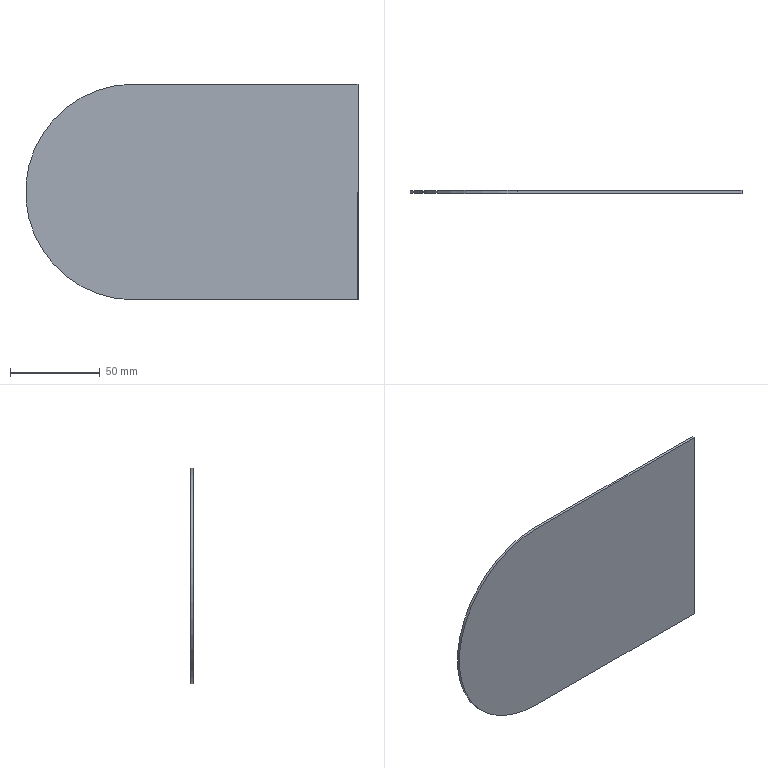Part | SolidWorks | features BaseBody 1 | 1 solid | 6 faces | box 185 x 1.5 x 120 mm | volume 30982 mm3 | plane 5 | cylinder 1 | commonest cylinder face diameters 120 x1
STEP:
#1=CARTESIAN_POINT('',(-62.5,0.,-60.));
#2=VERTEX_POINT('',#1);
#3=CARTESIAN_POINT('',(-62.5,0.,60.));
#4=VERTEX_POINT('',#3);
#5=CARTESIAN_POINT('',(-62.5,0.,0.));
#6=DIRECTION('',(0.,1.,0.));
#7=DIRECTION('',(0.,0.,1.));
#8=AXIS2_PLACEMENT_3D('',#5,#6,#7);
#9=CIRCLE('',#8,60.);
#10=EDGE_CURVE('',#2,#4,#9,.T.);
#11=ORIENTED_EDGE('',*,*,#10,.T.);
#12=CARTESIAN_POINT('',(62.5,0.,60.));
#13=VERTEX_POINT('',#12);
#14=CARTESIAN_POINT('',(-62.5,0.,60.));
#15=DIRECTION('',(1.,0.,0.));
#16=VECTOR('',#15,1000.);
#17=LINE('',#14,#16);
#18=EDGE_CURVE('',#4,#13,#17,.T.);
#19=ORIENTED_EDGE('',*,*,#18,.T.);
#20=CARTESIAN_POINT('',(62.5,0.,-60.));
#21=VERTEX_POINT('',#20);
#22=CARTESIAN_POINT('',(62.5,0.,0.));
#23=DIRECTION('',(0.,0.,-1.));
#24=VECTOR('',#23,1000.);
#25=LINE('',#22,#24);
#26=EDGE_CURVE('',#13,#21,#25,.T.);
#27=ORIENTED_EDGE('',*,*,#26,.T.);
#28=CARTESIAN_POINT('',(-62.5,0.,-60.));
#29=DIRECTION('',(-1.,0.,0.));
#30=VECTOR('',#29,1000.);
#31=LINE('',#28,#30);
#32=EDGE_CURVE('',#21,#2,#31,.T.);
#33=ORIENTED_EDGE('',*,*,#32,.T.);
#34=EDGE_LOOP('',(#11,#19,#27,#33));
#35=FACE_OUTER_BOUND('',#34,.T.);
#36=CARTESIAN_POINT('',(-62.5,0.,0.));
#37=DIRECTION('',(0.,1.,0.));
#38=DIRECTION('',(0.,0.,1.));
#39=AXIS2_PLACEMENT_3D('',#36,#37,#38);
#40=PLANE('',#39);
#41=ADVANCED_FACE('',(#35),#40,.T.);
#42=CARTESIAN_POINT('',(-62.5,-1.5,60.));
#43=VERTEX_POINT('',#42);
#44=CARTESIAN_POINT('',(62.5,-1.5,60.));
#45=VERTEX_POINT('',#44);
#46=CARTESIAN_POINT('',(-62.5,-1.5,60.));
#47=DIRECTION('',(1.,0.,0.));
#48=VECTOR('',#47,1000.);
#49=LINE('',#46,#48);
#50=EDGE_CURVE('',#43,#45,#49,.T.);
#51=ORIENTED_EDGE('',*,*,#50,.T.);
#52=CARTESIAN_POINT('',(62.5,-1.5,60.));
#53=DIRECTION('',(0.,1.,0.));
#54=VECTOR('',#53,1000.);
#55=LINE('',#52,#54);
#56=EDGE_CURVE('',#45,#13,#55,.T.);
#57=ORIENTED_EDGE('',*,*,#56,.T.);
#58=ORIENTED_EDGE('',*,*,#18,.F.);
#59=CARTESIAN_POINT('',(-62.5,-1.5,60.));
#60=DIRECTION('',(0.,-1.,0.));
#61=VECTOR('',#60,1000.);
#62=LINE('',#59,#61);
#63=EDGE_CURVE('',#4,#43,#62,.T.);
#64=ORIENTED_EDGE('',*,*,#63,.T.);
#65=EDGE_LOOP('',(#51,#57,#58,#64));
#66=FACE_OUTER_BOUND('',#65,.T.);
#67=CARTESIAN_POINT('',(-62.5,-1.5,60.));
#68=DIRECTION('',(0.,0.,1.));
#69=DIRECTION('',(1.,0.,0.));
#70=AXIS2_PLACEMENT_3D('',#67,#68,#69);
#71=PLANE('',#70);
#72=ADVANCED_FACE('',(#66),#71,.T.);
#73=CARTESIAN_POINT('',(-62.5,-1.5,-60.));
#74=VERTEX_POINT('',#73);
#75=CARTESIAN_POINT('',(-62.5,-1.5,0.));
#76=DIRECTION('',(0.,1.,0.));
#77=DIRECTION('',(0.,0.,1.));
#78=AXIS2_PLACEMENT_3D('',#75,#76,#77);
#79=CIRCLE('',#78,60.);
#80=EDGE_CURVE('',#74,#43,#79,.T.);
#81=ORIENTED_EDGE('',*,*,#80,.T.);
#82=ORIENTED_EDGE('',*,*,#63,.F.);
#83=ORIENTED_EDGE('',*,*,#10,.F.);
#84=CARTESIAN_POINT('',(-62.5,-1.5,-60.));
#85=DIRECTION('',(0.,-1.,0.));
#86=VECTOR('',#85,1000.);
#87=LINE('',#84,#86);
#88=EDGE_CURVE('',#2,#74,#87,.T.);
#89=ORIENTED_EDGE('',*,*,#88,.T.);
#90=EDGE_LOOP('',(#81,#82,#83,#89));
#91=FACE_OUTER_BOUND('',#90,.T.);
#92=CARTESIAN_POINT('',(-62.5,-1.5,0.));
#93=DIRECTION('',(0.,1.,0.));
#94=DIRECTION('',(0.,0.,1.));
#95=AXIS2_PLACEMENT_3D('',#92,#93,#94);
#96=CYLINDRICAL_SURFACE('',#95,60.);
#97=ADVANCED_FACE('',(#91),#96,.T.);
#98=CARTESIAN_POINT('',(62.5,-1.5,-60.));
#99=VERTEX_POINT('',#98);
#100=CARTESIAN_POINT('',(-62.5,-1.5,-60.));
#101=DIRECTION('',(-1.,0.,0.));
#102=VECTOR('',#101,1000.);
#103=LINE('',#100,#102);
#104=EDGE_CURVE('',#99,#74,#103,.T.);
#105=ORIENTED_EDGE('',*,*,#104,.T.);
#106=ORIENTED_EDGE('',*,*,#88,.F.);
#107=ORIENTED_EDGE('',*,*,#32,.F.);
#108=CARTESIAN_POINT('',(62.5,-1.5,-60.));
#109=DIRECTION('',(0.,-1.,0.));
#110=VECTOR('',#109,1000.);
#111=LINE('',#108,#110);
#112=EDGE_CURVE('',#21,#99,#111,.T.);
#113=ORIENTED_EDGE('',*,*,#112,.T.);
#114=EDGE_LOOP('',(#105,#106,#107,#113));
#115=FACE_OUTER_BOUND('',#114,.T.);
#116=CARTESIAN_POINT('',(-62.5,-1.5,-60.));
#117=DIRECTION('',(0.,0.,-1.));
#118=DIRECTION('',(-1.,0.,0.));
#119=AXIS2_PLACEMENT_3D('',#116,#117,#118);
#120=PLANE('',#119);
#121=ADVANCED_FACE('',(#115),#120,.T.);
#122=CARTESIAN_POINT('',(62.5,-1.5,60.));
#123=DIRECTION('',(0.,0.,-1.));
#124=VECTOR('',#123,1000.);
#125=LINE('',#122,#124);
#126=EDGE_CURVE('',#45,#99,#125,.T.);
#127=ORIENTED_EDGE('',*,*,#126,.T.);
#128=ORIENTED_EDGE('',*,*,#112,.F.);
#129=ORIENTED_EDGE('',*,*,#26,.F.);
#130=ORIENTED_EDGE('',*,*,#56,.F.);
#131=EDGE_LOOP('',(#127,#128,#129,#130));
#132=FACE_OUTER_BOUND('',#131,.T.);
#133=CARTESIAN_POINT('',(62.5,-1.5,60.));
#134=DIRECTION('',(1.,0.,0.));
#135=DIRECTION('',(0.,0.,-1.));
#136=AXIS2_PLACEMENT_3D('',#133,#134,#135);
#137=PLANE('',#136);
#138=ADVANCED_FACE('',(#132),#137,.T.);
#139=ORIENTED_EDGE('',*,*,#50,.F.);
#140=ORIENTED_EDGE('',*,*,#80,.F.);
#141=ORIENTED_EDGE('',*,*,#104,.F.);
#142=ORIENTED_EDGE('',*,*,#126,.F.);
#143=EDGE_LOOP('',(#139,#140,#141,#142));
#144=FACE_OUTER_BOUND('',#143,.T.);
#145=CARTESIAN_POINT('',(-62.5,-1.5,0.));
#146=DIRECTION('',(0.,1.,0.));
#147=DIRECTION('',(0.,0.,1.));
#148=AXIS2_PLACEMENT_3D('',#145,#146,#147);
#149=PLANE('',#148);
#150=ADVANCED_FACE('',(#144),#149,.F.);
#151=CLOSED_SHELL('',(#41,#72,#97,#121,#138,#150));
#152=MANIFOLD_SOLID_BREP('',#151);
#153=CARTESIAN_POINT('',(0.,0.,0.));
#154=DIRECTION('',(0.,0.,1.));
#155=DIRECTION('',(1.,0.,0.));
#156=AXIS2_PLACEMENT_3D('',#153,#154,#155);
#157=(LENGTH_UNIT()NAMED_UNIT(*)SI_UNIT(.MILLI.,.METRE.));
#158=UNCERTAINTY_MEASURE_WITH_UNIT(LENGTH_MEASURE(0.00001),#157,'','');
#159=(NAMED_UNIT(*)PLANE_ANGLE_UNIT()SI_UNIT($,.RADIAN.));
#160=(NAMED_UNIT(*)SI_UNIT($,.STERADIAN.)SOLID_ANGLE_UNIT());
#161=(GEOMETRIC_REPRESENTATION_CONTEXT(3)GLOBAL_UNCERTAINTY_ASSIGNED_CONTEXT((#158))GLOBAL_UNIT_ASSIGNED_CONTEXT((#157,#159,#160))REPRESENTATION_CONTEXT('',''));
#162=ADVANCED_BREP_SHAPE_REPRESENTATION('',(#152,#156),#161);